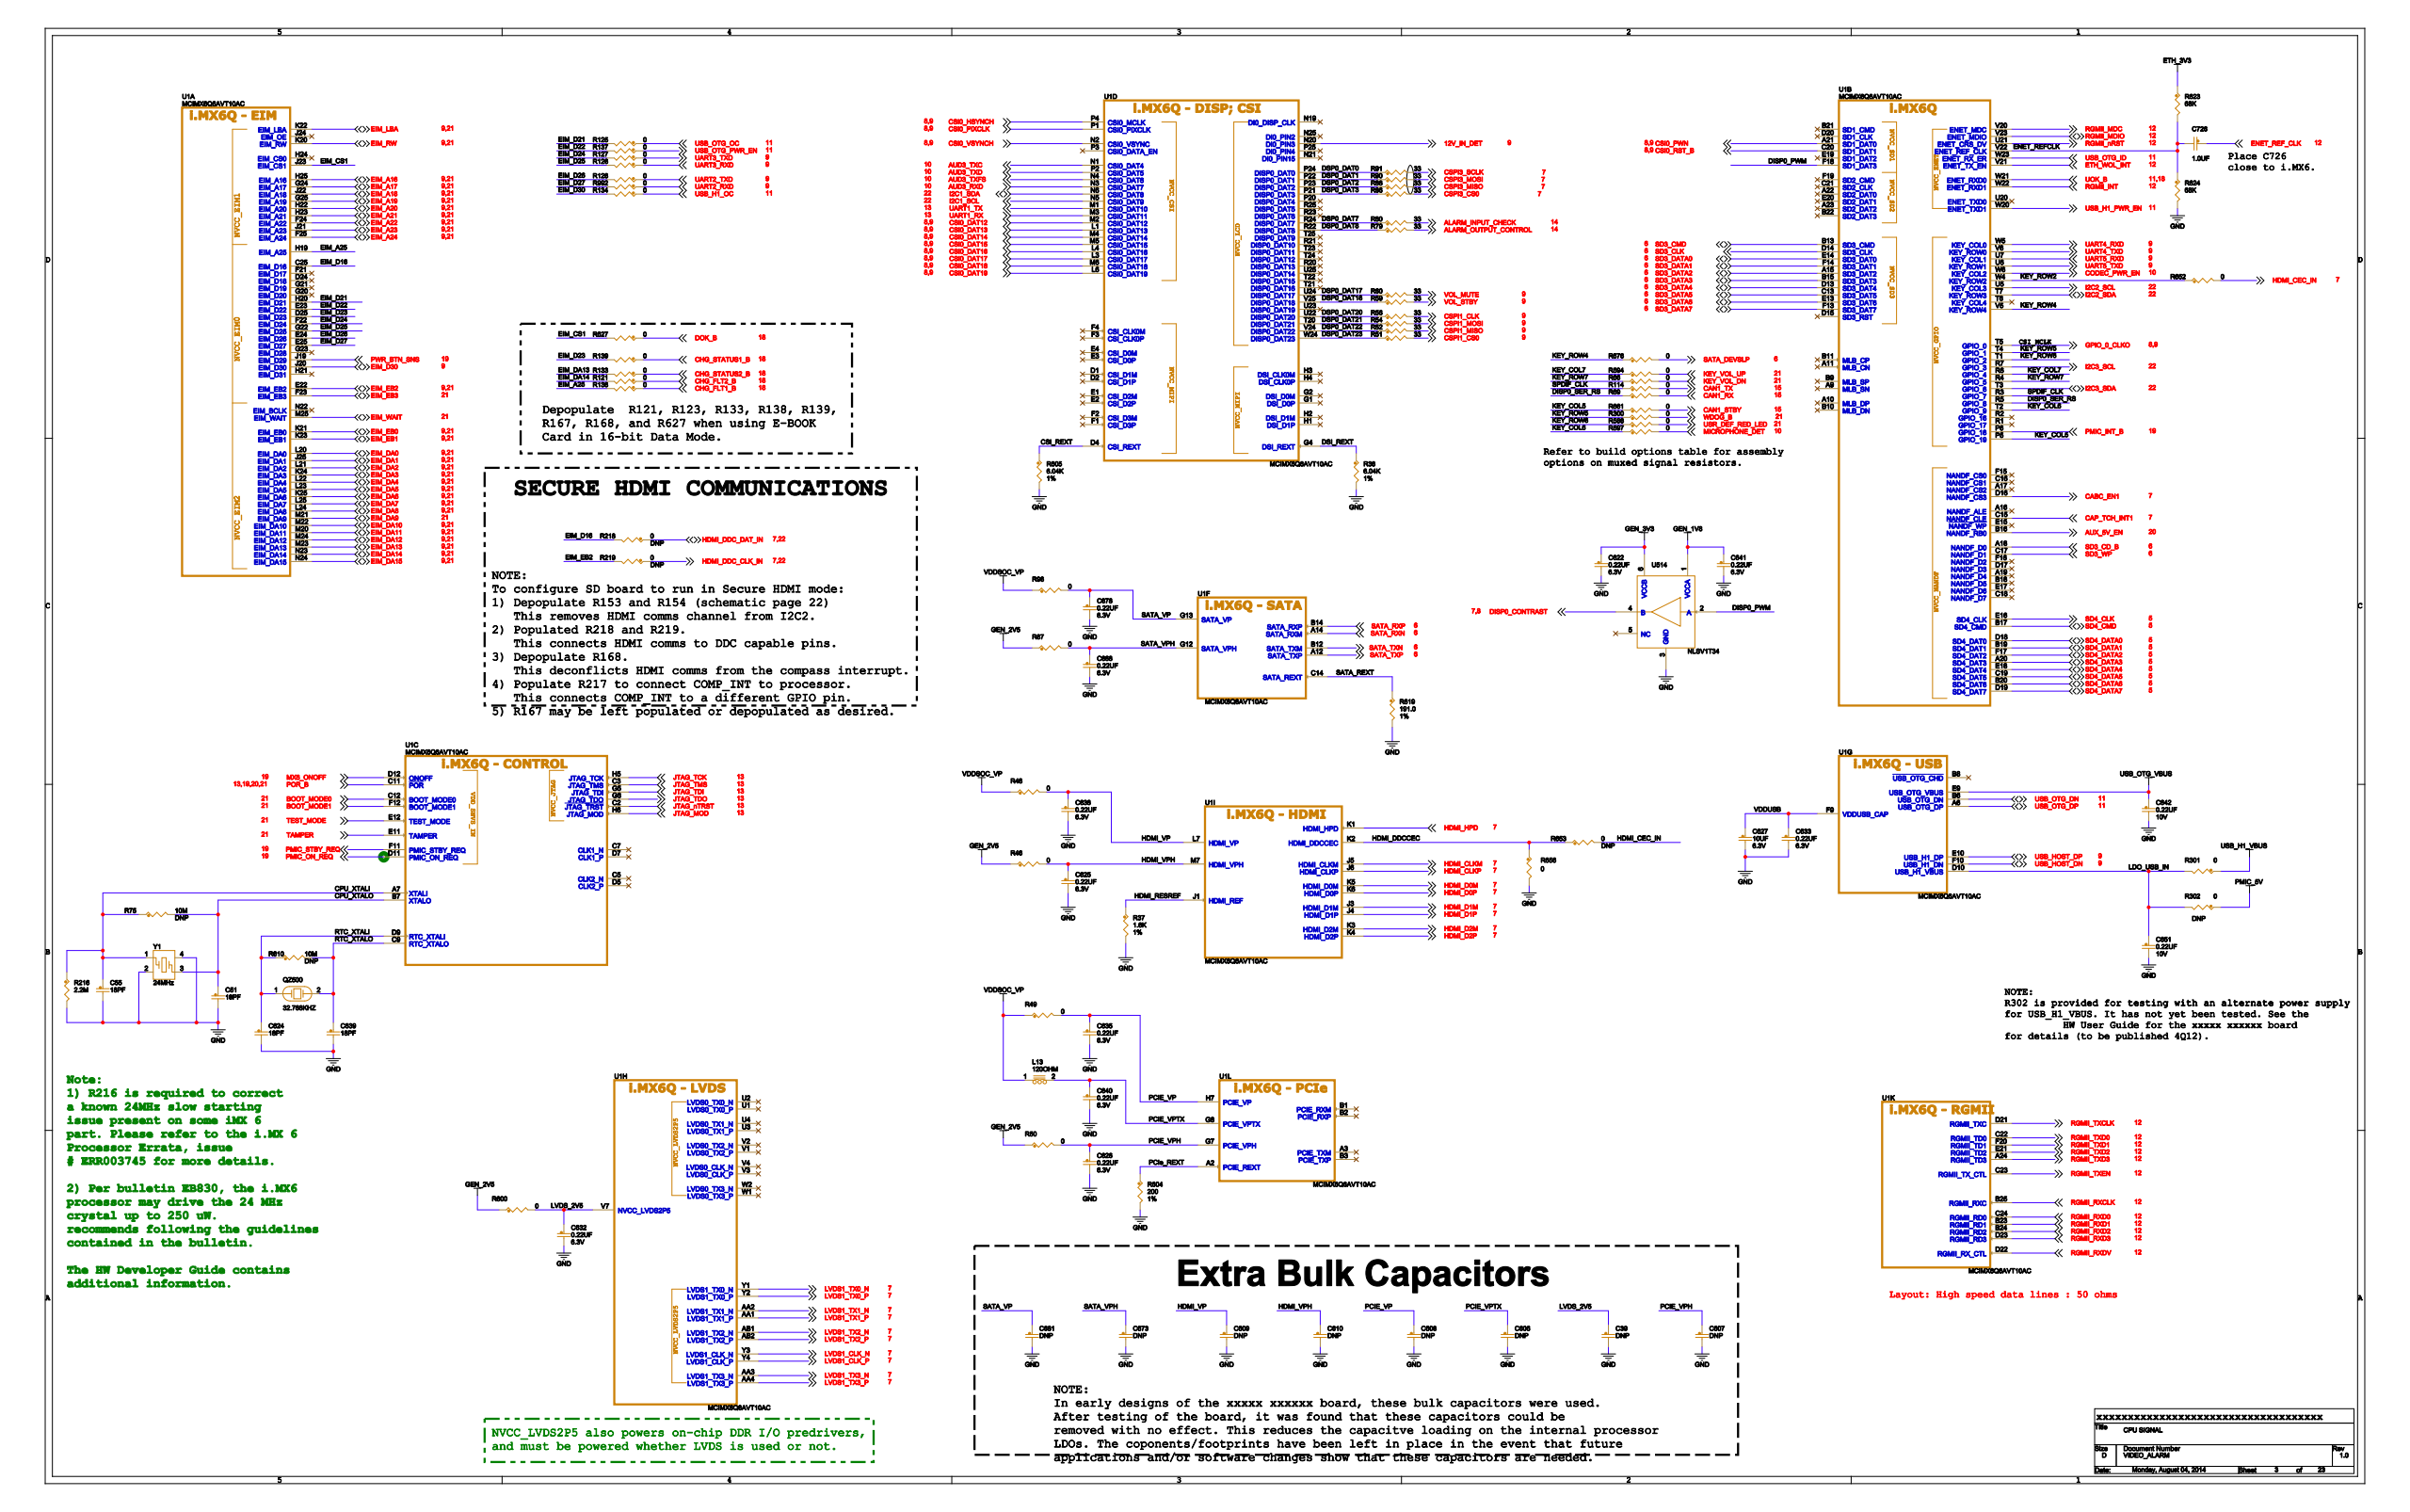Circuit board | Cadence Allegro | 994 parts | 728 nets | one sheet of the schematic
Parts on this sheet (reference | value | footprint):
C39 | 4.7uF | 0603_CC
C51 | 18PF | 0402_CC
C55 | 18PF | 0402_CC
C606 | 4.7UF | 0603_CC
C607 | 4.7UF | 0603_CC
C608 | 4.7UF | 0603_CC
C609 | 4.7UF | 0603_CC
C610 | 4.7UF | 0603_CC
C622 | 0.22UF | 0402_CC
C624 | 18PF | 0402_CC
C625 | 0.22UF | 0201_CC
C626 | 0.22UF | 0201_CC
C627 | 10UF | 0603_CC
C632 | 0.22UF | 0201_CC
C633 | 0.22UF | 0201_CC
C635 | 0.22UF | 0201_CC
C638 | 0.22UF | 0201_CC
C639 | 18PF | 0402_CC
C640 | 0.22UF | 0201_CC
C641 | 0.22UF | 0201_CC
C642 | 0.22UF | 0201_CC
C651 | 0.22UF | 0201_CC
C668 | 0.22UF | 0201_CC
C673 | 4.7UF | 0603_CC
C678 | 0.22UF | 0201_CC
C681 | 4.7UF | 0603_CC
C726 | 1.0UF | 0402_CC
L13 | 120OHM | 0603_CC
QZ500 | 32.768KHZ | XTAL2-3P2X1P5-SM
R37 | 1.6K | 0402_CC
R38 | 6.04K | 0402_CC
R46 | 0 | 0402_CC
R48 | 0 | 0402_CC
R49 | 0 | 0402_CC
R50 | 0 | 0402_CC
R51 | 33 | 0402_CC
R52 | 33 | 0402_CC
R54 | 33 | 0402_CC
R56 | 33 | 0402_CC
R59 | 33 | 0402_CC
R60 | 33 | 0402_CC
R66 | 0 | 0402_CC
R69 | 0 | 0402_CC
R75 | 10M | 0603_CC
R79 | 33 | 0402_CC
R80 | 33 | 0402_CC
R86 | 33 | 0402_CC
R87 | 0 | 0402_CC
R88 | 33 | 0402_CC
R90 | 33 | 0402_CC
R91 | 33 | 0402_CC
R96 | 0 | 0402_CC
R114 | 0 | 0402_CC
R121 | 0 | 0402_CC
R125 | 0 | 0402_CC
R126 | 0 | 0402_CC
R127 | 0 | 0402_CC
R128 | 0 | 0402_CC
R133 | 0 | 0402_CC
R134 | 0 | 0402_CC
R137 | 0 | 0402_CC
R138 | 0 | 0402_CC
R139 | 0 | 0402_CC
R216 | 2.2M | 0603_CC
R218 | 0 | 0402_CC
R219 | 0 | 0402_CC
R300 | 0 | 0402_CC
R301 | 0 | 0402_CC
R302 | 0 | 0402_CC
R588 | 0 | 0402_CC
R594 | 0 | 0402_CC
R597 | 0 | 0402_CC
R600 | 0 | 0402_CC
R604 | 200 | 0402_CC
R605 | 6.04K | 0402_CC
R610 | 10M | 0603_CC
R619 | 191.0 | 0603_CC
R623 | 68K | 0402_CC
R624 | 68K | 0402_CC
R627 | 0 | 0402_CC
R652 | 0 | 0402_CC
R653 | 0 | 0402_CC
R656 | 0 | 0402_CC
R661 | 0 | 0402_CC
R676 | 0 | 0402_CC
R992 | 0 | 0402_CC
U1 | MCIMX6Q6AVT10AC | BGA624_0P8_21X21
U2 | MT41K128M16JT | BGA96_0P8_8P15X14P15
U3 | MT41K128M16JT | BGA96_0P8_8P15X14P15
U4 | MT41K128M16JT | BGA96_0P8_8P15X14P15
U5 | MT41K128M16JT | BGA96_0P8_8P15X14P15
U7 | WM8962 | BGA49_0P5_3P62X4
U514 | NLSV1T34 | ULLGA6_1P45X1_0P5MM
Y1 | 24MHz | XTAL4_SX_3225
Nets of these parts (net: part-pin ...):
GND: C39-2 C51-2 C55-2 C606-2 C607-2 C608-2 C609-2 C610-2 C622-2 C624-2 C625-2 C626-2 C627-2 C632-2 C633-2 C635-2 C638-2 C639-2 C640-2 C641-2 C642-2 C651-2 C668-2 C673-2 C678-2 C681-2 R37-2 R38-2 R216-2 R604-2 R605-2 R619-2 R624-2 R656-2 U514-3 Y1-2 Y1-4 U2-A9 U2-B1 U2-B3 U2-B9 U2-D1 U2-E1 U2-E2 U2-F9 U2-G1 U2-G8 U2-M1 U2-P1 U2-T1 U3-A9 U3-B1 U3-B3 U3-B9 U3-D1 U3-E1 U3-E2 U3-F9 U3-G1 U3-G8 U3-M1 U3-P1 U3-T1 U4-A9 U4-B1 U4-B3 U4-B9 U4-D1 U4-E1 U4-E2 U4-F9 U4-G1 U4-G8 U4-M1 U4-P1 U4-T1 U5-A9 U5-B1 U5-B3 U5-B9 U5-D1 U5-E1 U5-E2 U5-F9 U5-G1 U5-G8 U5-M1 U5-P1 U5-T1 U7-F2 U7-F3 U7-G5
PMIC_INT_B: U1-P6
POR_B: U1-C11
PMIC_STBY_REQ: U1-F11
GEN_3V3: C622-1 U514-6
GEN_1V8: C641-1 U514-1
PMIC_5V: R302-1
PMIC_ON_REQ: U1-D11
UART4_RXD: U1-W5
UART5_TXD: U1-U6
UART4_TXD: U1-V6
UART5_RXD: U1-U7
CSI0_RST_B: U1-C20
CSI0_VSYNCH: U1-N2
CSI0_PWN: U1-A21
CSI0_HSYNCH: U1-P4
CSI0_DAT19: U1-L6
CSI0_DAT18: U1-M6
CSI0_DAT17: U1-L3
CSI0_DAT16: U1-L4
CSI0_DAT12: U1-M2
CSI0_DAT15: U1-M5
CSI0_DAT13: U1-L1
CSI0_DAT14: U1-M4
MX6_ONOFF: U1-D12
KEY_VOL_UP: R594-2
KEY_VOL_DN: R66-2
UART1_RX: U1-M3
UART1_TX: U1-M1
USB_OTG_ID: U1-W23
CSPI3_SCLK: R91-2
CSPI3_MISO: R88-2
CSPI3_MOSI: R90-2
CSPI3_CS0: R86-2
I2C1_SDA: U1-N6
I2C1_SCL: U1-N5
I2C2_SCL: U1-U5
I2C2_SDA: U1-T7
CABC_EN1: U1-D16
DISP0_CONTRAST: U514-4
CAP_TCH_INT1: U1-C15
HDMI_D0M: U1-K5
HDMI_CLKP: U1-J6
HDMI_CLKM: U1-J5
HDMI_D2M: U1-K3
HDMI_D1P: U1-J4
HDMI_D1M: U1-J3
HDMI_D0P: U1-K6
HDMI_D2P: U1-K4
UART2_RXD: R992-1
UART2_TXD: R128-1
UART3_RXD: R126-1
UART3_TXD: R127-1
ETH_3V3: R623-1
RGMII_MDIO: U1-V23
ALARM_INPUT_CHECK: R80-2
CPU_XTALI: C55-1 R75-1 R216-1 Y1-1 U1-A7
CPU_XTALO: C51-1 R75-2 Y1-3 U1-B7
RTC_XTALI: C624-1 QZ500-1 R610-1 U1-D9
RTC_XTALO: C639-1 QZ500-2 R610-2 U1-C9
HDMI_CEC_IN: R652-2 R653-2
HDMI_HPD: U1-K1
USB_OTG_OC: R125-1
USB_H1_OC: R134-1
CSI0_PIXCLK: U1-P1
EIM_D30: R134-2 U1-J20
USB_OTG_PWR_EN: R137-1
RGMII_RXCLK: U1-B25
SD3_CD_B: U1-A18
AUD3_TXD: U1-P2
AUD3_RXD: U1-N3
HDMI_DDC_CLK_IN: R219-1
HDMI_DDC_DAT_IN: R218-1
AUD3_TXFS: U1-N4
BOOT_MODE0: U1-C12
I2C3_SDA: U1-T3
I2C3_SCL: U1-R7
SATA_DEVSLP: R676-2
TAMPER: U1-E11
MICROPHONE_DET: R597-2
TEST_MODE: U1-E12
CODEC_PWR_EN: U1-W6
SD3_WP: U1-C17
SD3_CMD: U1-B13
SD3_DATA3: U1-B15
RGMII_RXD1: U1-B23
RGMII_RXD0: U1-C24
RGMII_RXD3: U1-D23
JTAG_TDO: U1-G6
JTAG_TCK: U1-H5
JTAG_TMS: U1-C3
JTAG_TDI: U1-G5
UOK_B: U1-W21
CHG_FLT2_B: R121-1
CHG_FLT1_B: R138-1
CHG_STATUS2_B: R133-1
CHG_STATUS1_B: R139-1
DOK_B: R627-1
SD4_CMD: U1-B17
ETH_WOL_INT: U1-V21
RGMII_INT: U1-W22
RGMII_RXDV: U1-D22
RGMII_RXD2: U1-B24
SD3_DATA4: U1-D13
SD3_DATA6: U1-E13
SD3_DATA7: U1-F13
SD3_DATA5: U1-C13
SD3_DATA2: U1-A15
SD3_CLK: U1-D14
SD3_DATA0: U1-E14
SD3_DATA1: U1-F14
BOOT_MODE1: U1-F12
SATA_TXP: U1-A12
SATA_TXN: U1-B12
SATA_RXN: U1-A14
SATA_RXP: U1-B14
AUX_5V_EN: U1-B16
CAN1_STBY: R661-2
CAN1_TX: R114-2
RGMII_TXCLK: U1-D21
RGMII_MDC: U1-V20
RGMII_TXD0: U1-C22
RGMII_TXD1: U1-F20
RGMII_TXD2: U1-E21
RGMII_TXD3: U1-A24
RGMII_TXEN: U1-C23
USB_H1_PWR_EN: U1-W20
USB_H1_VBUS: R301-1
SD4_CLK: U1-E16
SD4_DATA0: U1-D18
SD4_DATA1: U1-B19
SD4_DATA2: U1-F17
SD4_DATA3: U1-A20
SD4_DATA4: U1-E18
SD4_DATA5: U1-C19
SD4_DATA6: U1-B20
SD4_DATA7: U1-D19
CAN1_RX: R69-2
DISP0_PWM: U514-2 U1-F18
GPIO_0_CLKO: U1-T5
EIM_A16: U1-H25
EIM_A17: U1-G24
EIM_A18: U1-J22
EIM_A19: U1-G25
EIM_A20: U1-H22
EIM_A21: U1-H23
EIM_A22: U1-F24
EIM_A23: U1-J21
EIM_A24: U1-F25
EIM_A25: R138-2 U1-H19
EIM_CS1: R627-2 U1-J23
EIM_D16: R218-2 U1-C25
EIM_D21: R125-2 U1-H20
EIM_D22: R137-2 U1-E23
EIM_D23: R139-2 U1-D25
EIM_D24: R127-2 U1-F22
EIM_D25: R126-2 U1-G22
EIM_D26: R128-2 U1-E24
EIM_D27: R992-2 U1-E25
PWR_BTN_SNS: U1-J19
EIM_DA0: U1-L20
EIM_DA1: U1-J25
EIM_DA10: U1-M22
EIM_DA11: U1-M20
EIM_DA12: U1-M24
EIM_DA13: R133-2 U1-M23
EIM_DA14: R121-2 U1-N23
EIM_DA15: U1-N24
EIM_DA2: U1-L21
EIM_DA3: U1-K24
EIM_DA4: U1-L22
EIM_DA5: U1-L23
EIM_DA6: U1-K25
EIM_DA7: U1-L25
EIM_DA8: U1-L24
EIM_DA9: U1-M21
EIM_EB0: U1-K21
EIM_EB1: U1-K23
EIM_EB2: R219-2 U1-E22
EIM_EB3: U1-F23
EIM_LBA: U1-K22
EIM_RW: U1-K20
EIM_WAIT: U1-M25
ENET_REFCLK: C726-2 R623-2 R624-1 U1-V22
KEY_ROW5: R300-1 U1-T4
KEY_COL5: R661-1 U1-P5
KEY_ROW6: R588-1 U1-T1
KEY_COL7: R594-1 U1-R6
KEY_ROW7: R66-1 U1-R4
SPDIF_CLK: R114-1 U1-R3
DISP0_SER_RS: R69-1 U1-R5
KEY_COL6: R597-1 U1-T2
KEY_ROW2: R652-1 U1-W4
KEY_ROW4: R676-1 U1-V5
JTAG_MOD: U1-H6
AUD3_TXC: U1-N1
CSI_REXT: R605-1 U1-D4
12V_IN_DET: U1-N20
DSP0_DAT0: R91-1 U1-P24
DSP0_DAT1: R90-1 U1-P22
DSP0_DAT17: R60-1 U1-U24
DSP0_DAT18: R59-1 U1-V25
DSP0_DAT2: R88-1 U1-P23
DSP0_DAT20: R56-1 U1-U22
DSP0_DAT21: R54-1 U1-T20
DSP0_DAT22: R52-1 U1-V24
DSP0_DAT23: R51-1 U1-W24
DSP0_DAT3: R86-1 U1-P21
DSP0_DAT7: R80-1 U1-R24
DSP0_DAT8: R79-1 U1-R22
DSI_REXT: R38-1 U1-G4
SATA_REXT: R619-1 U1-C14
SATA_VP: C678-1 C681-1 R96-2 U1-G13
SATA_VPH: C668-1 C673-1 R87-2 U1-G12
USB_HOST_DN: U1-F10
USB_HOST_DP: U1-E10
LDO_USB_IN: C651-1 R301-2 R302-2 U1-D10
USB_OTG_DN: U1-B6
USB_OTG_DP: U1-A6
USB_OTG_VBUS: C642-1 U1-E9
VDDUSB: C627-1 C633-1 U1-F9
LVDS1_CLK_N: U1-Y3
LVDS1_CLK_P: U1-Y4
LVDS1_TX0_N: U1-Y1
LVDS1_TX0_P: U1-Y2
LVDS1_TX1_N: U1-AA2
LVDS1_TX1_P: U1-AA1
LVDS1_TX2_N: U1-AB1
LVDS1_TX2_P: U1-AB2
LVDS1_TX3_N: U1-AA3
LVDS1_TX3_P: U1-AA4
LVDS_2V5: C39-1 C632-1 R600-2 U1-V7
HDMI_DDCCEC: R653-1 R656-1 U1-K2
HDMI_RESREF: R37-1 U1-J1
HDMI_VP: C609-1 C638-1 R48-2 U1-L7
HDMI_VPH: C610-1 C625-1 R46-2 U1-M7
PCIE_REXT: R604-1 U1-A2
PCIE_VP: C608-1 C635-1 R49-2 U1-H7
PCIE_VPH: C607-1 C626-1 R50-2 U1-G7
PCIE_VPTX: C606-1 C640-1 L13-2 U1-G8
USR_DEF_RED_LED: R588-2
ALARM_OUTPUT_CONTROL: R79-2
VOL_STBY: R59-2
VOL_MUTE: R60-2
GEN_2V5: R46-1 R50-1 R87-1 R600-1
CSPI1_CS0: R51-2
CSPI1_MISO: R52-2
CSPI1_MOSI: R54-2
CSPI1_CLK: R56-2
VDDSOC_VP: L13-1 R48-1 R49-1 R96-1
WDOG_B: R300-2
ENET_REF_CLK: C726-1